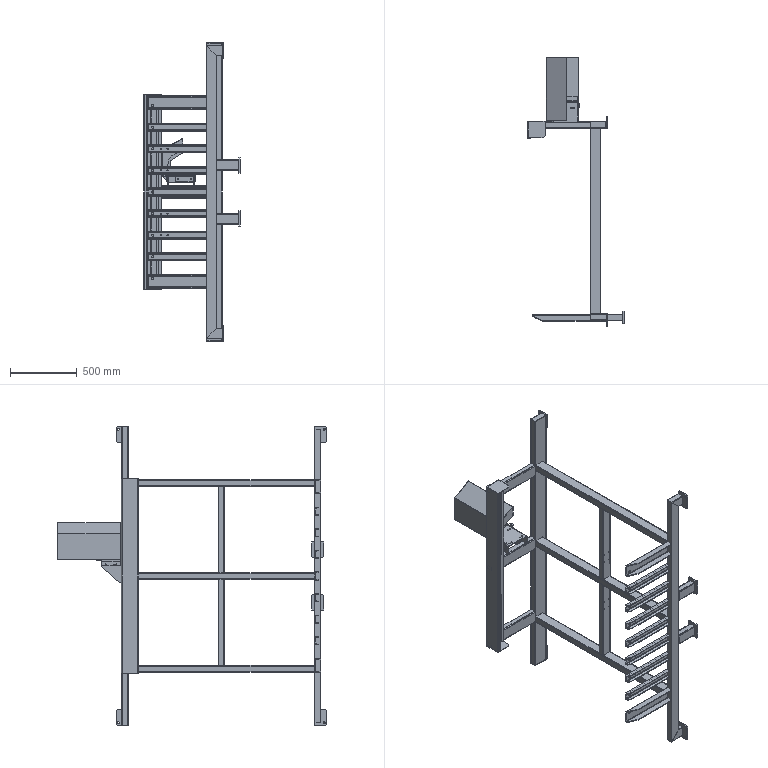Part | SolidWorks | 55 solids | 886 faces | box 723.5 x 2013 x 2240 mm | volume 19129851 mm3 | plane 549 | cylinder 337 | commonest cylinder face diameters 10 x52 8 x46 17 x38 6 x35 4 x30 2 x28